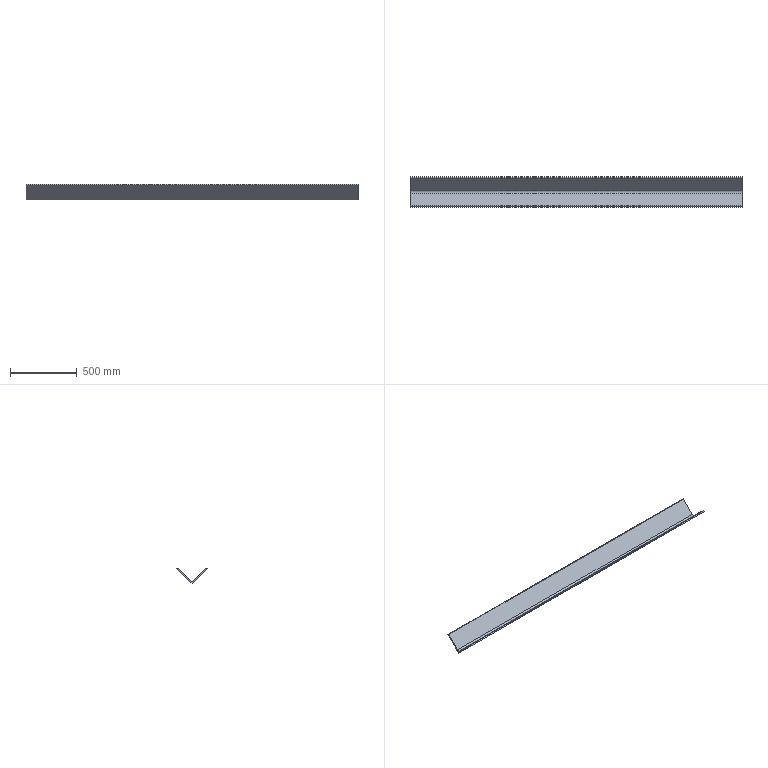Part | STEP file | Angle steel L160X60X10-2484_Default<As machined> | 1 solid | 13 faces | box 2484 x 226.274 x 118.827 mm | volume 7825020 mm3 | plane 8 | cylinder 5 | commonest cylinder face diameters 6.667 x4 32 x1
STEP:
#1=CARTESIAN_POINT('',(0.,0.,0.));
#2=DIRECTION('',(0.,0.,1.));
#3=DIRECTION('',(1.,0.,0.));
#4=AXIS2_PLACEMENT_3D('',#1,#2,#3);
#5=CARTESIAN_POINT('',(1242.,-106.066,118.827));
#6=VERTEX_POINT('',#5);
#7=CARTESIAN_POINT('',(1242.,-108.423,117.851));
#8=VERTEX_POINT('',#7);
#9=CARTESIAN_POINT('',(1242.,-106.066,115.494));
#10=DIRECTION('',(1.,0.,0.));
#11=DIRECTION('',(0.,0.,1.));
#12=AXIS2_PLACEMENT_3D('',#9,#10,#11);
#13=CIRCLE('',#12,3.333);
#14=CARTESIAN_POINT('',(1242.,-106.066,115.494));
#15=DIRECTION('',(-1.,0.,0.));
#16=DIRECTION('',(0.,0.,1.));
#17=AXIS2_PLACEMENT_3D('',#14,#15,#16);
#18=CYLINDRICAL_SURFACE('',#17,3.333);
#19=CARTESIAN_POINT('',(6.283,0.));
#20=DIRECTION('',(-1.,0.));
#21=VECTOR('',#20,1.);
#22=LINE('',#19,#21);
#23=(GEOMETRIC_REPRESENTATION_CONTEXT(2)PARAMETRIC_REPRESENTATION_CONTEXT()REPRESENTATION_CONTEXT('',''));
#24=DEFINITIONAL_REPRESENTATION('',(#22),#23);
#25=PCURVE('',#18,#24);
#26=CARTESIAN_POINT('',(1242.,-106.066,115.494));
#27=DIRECTION('',(-1.,0.,0.));
#28=DIRECTION('',(0.,0.,1.));
#29=AXIS2_PLACEMENT_3D('',#26,#27,#28);
#30=PLANE('',#29);
#31=CARTESIAN_POINT('',(3.333,0.));
#32=CARTESIAN_POINT('',(3.333,-5.774));
#33=CARTESIAN_POINT('',(-1.667,-2.887));
#34=CARTESIAN_POINT('',(-6.667,0.));
#35=CARTESIAN_POINT('',(-1.667,2.887));
#36=CARTESIAN_POINT('',(3.333,5.774));
#37=CARTESIAN_POINT('',(3.333,0.));
#38=(BOUNDED_CURVE()B_SPLINE_CURVE(2,(#31,#32,#33,#34,#35,#36,#37),.UNSPECIFIED.,.T.,.F.)B_SPLINE_CURVE_WITH_KNOTS((1,2,2,2,2,1),(-2.094,0.,2.094,4.189,6.283,8.378),.UNSPECIFIED.)CURVE()GEOMETRIC_REPRESENTATION_ITEM()RATIONAL_B_SPLINE_CURVE((1.,0.5,1.,0.5,1.,0.5,1.))REPRESENTATION_ITEM(''));
#39=(GEOMETRIC_REPRESENTATION_CONTEXT(2)PARAMETRIC_REPRESENTATION_CONTEXT()REPRESENTATION_CONTEXT('',''));
#40=DEFINITIONAL_REPRESENTATION('',(#38),#39);
#41=PCURVE('',#30,#40);
#42=SURFACE_CURVE('',#13,(#25,#41),.PCURVE_S1.);
#43=EDGE_CURVE('',#6,#8,#42,.T.);
#44=ORIENTED_EDGE('',*,*,#43,.F.);
#45=CARTESIAN_POINT('',(-1242.,-106.066,118.827));
#46=VERTEX_POINT('',#45);
#47=CARTESIAN_POINT('',(1242.,-106.066,118.827));
#48=DIRECTION('',(-1.,0.,0.));
#49=VECTOR('',#48,1.);
#50=LINE('',#47,#49);
#51=CARTESIAN_POINT('',(6.283,0.));
#52=DIRECTION('',(0.,1.));
#53=VECTOR('',#52,1.);
#54=LINE('',#51,#53);
#55=(GEOMETRIC_REPRESENTATION_CONTEXT(2)PARAMETRIC_REPRESENTATION_CONTEXT()REPRESENTATION_CONTEXT('',''));
#56=DEFINITIONAL_REPRESENTATION('',(#54),#55);
#57=PCURVE('',#18,#56);
#58=CARTESIAN_POINT('',(1242.,-106.066,115.494));
#59=DIRECTION('',(-1.,0.,0.));
#60=DIRECTION('',(0.,0.,1.));
#61=AXIS2_PLACEMENT_3D('',#58,#59,#60);
#62=CYLINDRICAL_SURFACE('',#61,3.333);
#63=CARTESIAN_POINT('',(0.,0.));
#64=DIRECTION('',(0.,1.));
#65=VECTOR('',#64,1.);
#66=LINE('',#63,#65);
#67=(GEOMETRIC_REPRESENTATION_CONTEXT(2)PARAMETRIC_REPRESENTATION_CONTEXT()REPRESENTATION_CONTEXT('',''));
#68=DEFINITIONAL_REPRESENTATION('',(#66),#67);
#69=PCURVE('',#62,#68);
#70=SURFACE_CURVE('',#50,(#57,#69),.PCURVE_S1.);
#71=EDGE_CURVE('',#6,#46,#70,.T.);
#72=ORIENTED_EDGE('',*,*,#71,.T.);
#73=CARTESIAN_POINT('',(-1242.,-108.423,117.851));
#74=VERTEX_POINT('',#73);
#75=CARTESIAN_POINT('',(-1242.,-106.066,115.494));
#76=DIRECTION('',(1.,0.,0.));
#77=DIRECTION('',(0.,0.,1.));
#78=AXIS2_PLACEMENT_3D('',#75,#76,#77);
#79=CIRCLE('',#78,3.333);
#80=CARTESIAN_POINT('',(6.283,2484.));
#81=DIRECTION('',(-1.,0.));
#82=VECTOR('',#81,1.);
#83=LINE('',#80,#82);
#84=(GEOMETRIC_REPRESENTATION_CONTEXT(2)PARAMETRIC_REPRESENTATION_CONTEXT()REPRESENTATION_CONTEXT('',''));
#85=DEFINITIONAL_REPRESENTATION('',(#83),#84);
#86=PCURVE('',#18,#85);
#87=CARTESIAN_POINT('',(-1242.,-106.066,115.494));
#88=DIRECTION('',(-1.,0.,0.));
#89=DIRECTION('',(0.,0.,1.));
#90=AXIS2_PLACEMENT_3D('',#87,#88,#89);
#91=PLANE('',#90);
#92=CARTESIAN_POINT('',(3.333,0.));
#93=CARTESIAN_POINT('',(3.333,-5.774));
#94=CARTESIAN_POINT('',(-1.667,-2.887));
#95=CARTESIAN_POINT('',(-6.667,0.));
#96=CARTESIAN_POINT('',(-1.667,2.887));
#97=CARTESIAN_POINT('',(3.333,5.774));
#98=CARTESIAN_POINT('',(3.333,0.));
#99=(BOUNDED_CURVE()B_SPLINE_CURVE(2,(#92,#93,#94,#95,#96,#97,#98),.UNSPECIFIED.,.T.,.F.)B_SPLINE_CURVE_WITH_KNOTS((1,2,2,2,2,1),(-2.094,0.,2.094,4.189,6.283,8.378),.UNSPECIFIED.)CURVE()GEOMETRIC_REPRESENTATION_ITEM()RATIONAL_B_SPLINE_CURVE((1.,0.5,1.,0.5,1.,0.5,1.))REPRESENTATION_ITEM(''));
#100=(GEOMETRIC_REPRESENTATION_CONTEXT(2)PARAMETRIC_REPRESENTATION_CONTEXT()REPRESENTATION_CONTEXT('',''));
#101=DEFINITIONAL_REPRESENTATION('',(#99),#100);
#102=PCURVE('',#91,#101);
#103=SURFACE_CURVE('',#79,(#86,#102),.PCURVE_S1.);
#104=EDGE_CURVE('',#46,#74,#103,.T.);
#105=ORIENTED_EDGE('',*,*,#104,.T.);
#106=CARTESIAN_POINT('',(1242.,-108.423,117.851));
#107=DIRECTION('',(-1.,0.,0.));
#108=VECTOR('',#107,1.);
#109=LINE('',#106,#108);
#110=CARTESIAN_POINT('',(5.498,0.));
#111=DIRECTION('',(0.,1.));
#112=VECTOR('',#111,1.);
#113=LINE('',#110,#112);
#114=(GEOMETRIC_REPRESENTATION_CONTEXT(2)PARAMETRIC_REPRESENTATION_CONTEXT()REPRESENTATION_CONTEXT('',''));
#115=DEFINITIONAL_REPRESENTATION('',(#113),#114);
#116=PCURVE('',#18,#115);
#117=CARTESIAN_POINT('',(1242.,-113.137,113.137));
#118=DIRECTION('',(0.,0.7071,-0.7071));
#119=DIRECTION('',(0.,0.7071,0.7071));
#120=AXIS2_PLACEMENT_3D('',#117,#118,#119);
#121=PLANE('',#120);
#122=CARTESIAN_POINT('',(6.667,0.));
#123=DIRECTION('',(0.,-1.));
#124=VECTOR('',#123,1.);
#125=LINE('',#122,#124);
#126=(GEOMETRIC_REPRESENTATION_CONTEXT(2)PARAMETRIC_REPRESENTATION_CONTEXT()REPRESENTATION_CONTEXT('',''));
#127=DEFINITIONAL_REPRESENTATION('',(#125),#126);
#128=PCURVE('',#121,#127);
#129=SURFACE_CURVE('',#109,(#116,#128),.PCURVE_S1.);
#130=EDGE_CURVE('',#8,#74,#129,.T.);
#131=ORIENTED_EDGE('',*,*,#130,.F.);
#132=EDGE_LOOP('',(#44,#72,#105,#131));
#133=FACE_BOUND('',#132,.T.);
#134=ADVANCED_FACE('',(#133),#18,.T.);
#135=CARTESIAN_POINT('',(1242.,106.066,118.827));
#136=VERTEX_POINT('',#135);
#137=CARTESIAN_POINT('',(1242.,103.709,117.851));
#138=VERTEX_POINT('',#137);
#139=CARTESIAN_POINT('',(1242.,106.066,115.494));
#140=DIRECTION('',(1.,0.,0.));
#141=DIRECTION('',(0.,0.,-1.));
#142=AXIS2_PLACEMENT_3D('',#139,#140,#141);
#143=CIRCLE('',#142,3.333);
#144=CARTESIAN_POINT('',(1242.,106.066,115.494));
#145=DIRECTION('',(-1.,0.,0.));
#146=DIRECTION('',(0.,0.,1.));
#147=AXIS2_PLACEMENT_3D('',#144,#145,#146);
#148=CYLINDRICAL_SURFACE('',#147,3.333);
#149=CARTESIAN_POINT('',(9.425,0.));
#150=DIRECTION('',(-1.,0.));
#151=VECTOR('',#150,1.);
#152=LINE('',#149,#151);
#153=(GEOMETRIC_REPRESENTATION_CONTEXT(2)PARAMETRIC_REPRESENTATION_CONTEXT()REPRESENTATION_CONTEXT('',''));
#154=DEFINITIONAL_REPRESENTATION('',(#152),#153);
#155=PCURVE('',#148,#154);
#156=CARTESIAN_POINT('',(-3.333,212.132));
#157=CARTESIAN_POINT('',(-3.333,217.906));
#158=CARTESIAN_POINT('',(1.667,215.019));
#159=CARTESIAN_POINT('',(6.667,212.132));
#160=CARTESIAN_POINT('',(1.667,209.245));
#161=CARTESIAN_POINT('',(-3.333,206.359));
#162=CARTESIAN_POINT('',(-3.333,212.132));
#163=(BOUNDED_CURVE()B_SPLINE_CURVE(2,(#156,#157,#158,#159,#160,#161,#162),.UNSPECIFIED.,.T.,.F.)B_SPLINE_CURVE_WITH_KNOTS((1,2,2,2,2,1),(-2.094,0.,2.094,4.189,6.283,8.378),.UNSPECIFIED.)CURVE()GEOMETRIC_REPRESENTATION_ITEM()RATIONAL_B_SPLINE_CURVE((1.,0.5,1.,0.5,1.,0.5,1.))REPRESENTATION_ITEM(''));
#164=(GEOMETRIC_REPRESENTATION_CONTEXT(2)PARAMETRIC_REPRESENTATION_CONTEXT()REPRESENTATION_CONTEXT('',''));
#165=DEFINITIONAL_REPRESENTATION('',(#163),#164);
#166=PCURVE('',#30,#165);
#167=SURFACE_CURVE('',#143,(#155,#166),.PCURVE_S1.);
#168=EDGE_CURVE('',#136,#138,#167,.T.);
#169=ORIENTED_EDGE('',*,*,#168,.F.);
#170=CARTESIAN_POINT('',(-1242.,106.066,118.827));
#171=VERTEX_POINT('',#170);
#172=CARTESIAN_POINT('',(1242.,106.066,118.827));
#173=DIRECTION('',(-1.,0.,0.));
#174=VECTOR('',#173,1.);
#175=LINE('',#172,#174);
#176=CARTESIAN_POINT('',(6.283,0.));
#177=DIRECTION('',(0.,1.));
#178=VECTOR('',#177,1.);
#179=LINE('',#176,#178);
#180=(GEOMETRIC_REPRESENTATION_CONTEXT(2)PARAMETRIC_REPRESENTATION_CONTEXT()REPRESENTATION_CONTEXT('',''));
#181=DEFINITIONAL_REPRESENTATION('',(#179),#180);
#182=PCURVE('',#148,#181);
#183=CARTESIAN_POINT('',(1242.,106.066,115.494));
#184=DIRECTION('',(-1.,0.,0.));
#185=DIRECTION('',(0.,0.,1.));
#186=AXIS2_PLACEMENT_3D('',#183,#184,#185);
#187=CYLINDRICAL_SURFACE('',#186,3.333);
#188=CARTESIAN_POINT('',(0.,0.));
#189=DIRECTION('',(0.,1.));
#190=VECTOR('',#189,1.);
#191=LINE('',#188,#190);
#192=(GEOMETRIC_REPRESENTATION_CONTEXT(2)PARAMETRIC_REPRESENTATION_CONTEXT()REPRESENTATION_CONTEXT('',''));
#193=DEFINITIONAL_REPRESENTATION('',(#191),#192);
#194=PCURVE('',#187,#193);
#195=SURFACE_CURVE('',#175,(#182,#194),.PCURVE_S1.);
#196=EDGE_CURVE('',#136,#171,#195,.T.);
#197=ORIENTED_EDGE('',*,*,#196,.T.);
#198=CARTESIAN_POINT('',(-1242.,103.709,117.851));
#199=VERTEX_POINT('',#198);
#200=CARTESIAN_POINT('',(-1242.,106.066,115.494));
#201=DIRECTION('',(1.,0.,0.));
#202=DIRECTION('',(0.,0.,-1.));
#203=AXIS2_PLACEMENT_3D('',#200,#201,#202);
#204=CIRCLE('',#203,3.333);
#205=CARTESIAN_POINT('',(9.425,2484.));
#206=DIRECTION('',(-1.,0.));
#207=VECTOR('',#206,1.);
#208=LINE('',#205,#207);
#209=(GEOMETRIC_REPRESENTATION_CONTEXT(2)PARAMETRIC_REPRESENTATION_CONTEXT()REPRESENTATION_CONTEXT('',''));
#210=DEFINITIONAL_REPRESENTATION('',(#208),#209);
#211=PCURVE('',#148,#210);
#212=CARTESIAN_POINT('',(-3.333,212.132));
#213=CARTESIAN_POINT('',(-3.333,217.906));
#214=CARTESIAN_POINT('',(1.667,215.019));
#215=CARTESIAN_POINT('',(6.667,212.132));
#216=CARTESIAN_POINT('',(1.667,209.245));
#217=CARTESIAN_POINT('',(-3.333,206.359));
#218=CARTESIAN_POINT('',(-3.333,212.132));
#219=(BOUNDED_CURVE()B_SPLINE_CURVE(2,(#212,#213,#214,#215,#216,#217,#218),.UNSPECIFIED.,.T.,.F.)B_SPLINE_CURVE_WITH_KNOTS((1,2,2,2,2,1),(-2.094,0.,2.094,4.189,6.283,8.378),.UNSPECIFIED.)CURVE()GEOMETRIC_REPRESENTATION_ITEM()RATIONAL_B_SPLINE_CURVE((1.,0.5,1.,0.5,1.,0.5,1.))REPRESENTATION_ITEM(''));
#220=(GEOMETRIC_REPRESENTATION_CONTEXT(2)PARAMETRIC_REPRESENTATION_CONTEXT()REPRESENTATION_CONTEXT('',''));
#221=DEFINITIONAL_REPRESENTATION('',(#219),#220);
#222=PCURVE('',#91,#221);
#223=SURFACE_CURVE('',#204,(#211,#222),.PCURVE_S1.);
#224=EDGE_CURVE('',#171,#199,#223,.T.);
#225=ORIENTED_EDGE('',*,*,#224,.T.);
#226=CARTESIAN_POINT('',(1242.,103.709,117.851));
#227=DIRECTION('',(-1.,0.,0.));
#228=VECTOR('',#227,1.);
#229=LINE('',#226,#228);
#230=CARTESIAN_POINT('',(5.498,0.));
#231=DIRECTION('',(0.,1.));
#232=VECTOR('',#231,1.);
#233=LINE('',#230,#232);
#234=(GEOMETRIC_REPRESENTATION_CONTEXT(2)PARAMETRIC_REPRESENTATION_CONTEXT()REPRESENTATION_CONTEXT('',''));
#235=DEFINITIONAL_REPRESENTATION('',(#233),#234);
#236=PCURVE('',#148,#235);
#237=CARTESIAN_POINT('',(1242.,11.314,25.456));
#238=DIRECTION('',(0.,0.7071,-0.7071));
#239=DIRECTION('',(0.,0.7071,0.7071));
#240=AXIS2_PLACEMENT_3D('',#237,#238,#239);
#241=PLANE('',#240);
#242=CARTESIAN_POINT('',(130.667,0.));
#243=DIRECTION('',(0.,-1.));
#244=VECTOR('',#243,1.);
#245=LINE('',#242,#244);
#246=(GEOMETRIC_REPRESENTATION_CONTEXT(2)PARAMETRIC_REPRESENTATION_CONTEXT()REPRESENTATION_CONTEXT('',''));
#247=DEFINITIONAL_REPRESENTATION('',(#245),#246);
#248=PCURVE('',#241,#247);
#249=SURFACE_CURVE('',#229,(#236,#248),.PCURVE_S1.);
#250=EDGE_CURVE('',#138,#199,#249,.T.);
#251=ORIENTED_EDGE('',*,*,#250,.F.);
#252=EDGE_LOOP('',(#169,#197,#225,#251));
#253=FACE_BOUND('',#252,.T.);
#254=ADVANCED_FACE('',(#253),#148,.T.);
#255=CARTESIAN_POINT('',(-1242.,0.,0.));
#256=VERTEX_POINT('',#255);
#257=CARTESIAN_POINT('',(-1242.,113.137,113.137));
#258=VERTEX_POINT('',#257);
#259=CARTESIAN_POINT('',(-1242.,113.137,113.137));
#260=DIRECTION('',(0.,0.7071,0.7071));
#261=VECTOR('',#260,1.);
#262=LINE('',#259,#261);
#263=CARTESIAN_POINT('',(1242.,113.137,113.137));
#264=DIRECTION('',(0.,-0.7071,0.7071));
#265=DIRECTION('',(0.,-0.7071,-0.7071));
#266=AXIS2_PLACEMENT_3D('',#263,#264,#265);
#267=PLANE('',#266);
#268=CARTESIAN_POINT('',(0.,-2484.));
#269=DIRECTION('',(-1.,0.));
#270=VECTOR('',#269,1.);
#271=LINE('',#268,#270);
#272=(GEOMETRIC_REPRESENTATION_CONTEXT(2)PARAMETRIC_REPRESENTATION_CONTEXT()REPRESENTATION_CONTEXT('',''));
#273=DEFINITIONAL_REPRESENTATION('',(#271),#272);
#274=PCURVE('',#267,#273);
#275=CARTESIAN_POINT('',(-2.357,219.203));
#276=DIRECTION('',(0.7071,0.7071));
#277=VECTOR('',#276,1.);
#278=LINE('',#275,#277);
#279=(GEOMETRIC_REPRESENTATION_CONTEXT(2)PARAMETRIC_REPRESENTATION_CONTEXT()REPRESENTATION_CONTEXT('',''));
#280=DEFINITIONAL_REPRESENTATION('',(#278),#279);
#281=PCURVE('',#91,#280);
#282=SURFACE_CURVE('',#262,(#274,#281),.PCURVE_S1.);
#283=EDGE_CURVE('',#256,#258,#282,.T.);
#284=ORIENTED_EDGE('',*,*,#283,.T.);
#285=CARTESIAN_POINT('',(1242.,113.137,113.137));
#286=VERTEX_POINT('',#285);
#287=CARTESIAN_POINT('',(1242.,113.137,113.137));
#288=DIRECTION('',(-1.,0.,0.));
#289=VECTOR('',#288,1.);
#290=LINE('',#287,#289);
#291=CARTESIAN_POINT('',(0.,0.));
#292=DIRECTION('',(0.,-1.));
#293=VECTOR('',#292,1.);
#294=LINE('',#291,#293);
#295=(GEOMETRIC_REPRESENTATION_CONTEXT(2)PARAMETRIC_REPRESENTATION_CONTEXT()REPRESENTATION_CONTEXT('',''));
#296=DEFINITIONAL_REPRESENTATION('',(#294),#295);
#297=PCURVE('',#267,#296);
#298=CARTESIAN_POINT('',(1242.,113.137,113.137));
#299=DIRECTION('',(0.,-0.7071,-0.7071));
#300=DIRECTION('',(0.,0.7071,-0.7071));
#301=AXIS2_PLACEMENT_3D('',#298,#299,#300);
#302=PLANE('',#301);
#303=CARTESIAN_POINT('',(0.,0.));
#304=DIRECTION('',(0.,-1.));
#305=VECTOR('',#304,1.);
#306=LINE('',#303,#305);
#307=(GEOMETRIC_REPRESENTATION_CONTEXT(2)PARAMETRIC_REPRESENTATION_CONTEXT()REPRESENTATION_CONTEXT('',''));
#308=DEFINITIONAL_REPRESENTATION('',(#306),#307);
#309=PCURVE('',#302,#308);
#310=SURFACE_CURVE('',#290,(#297,#309),.PCURVE_S1.);
#311=EDGE_CURVE('',#286,#258,#310,.T.);
#312=ORIENTED_EDGE('',*,*,#311,.F.);
#313=CARTESIAN_POINT('',(1242.,0.,0.));
#314=VERTEX_POINT('',#313);
#315=CARTESIAN_POINT('',(1242.,113.137,113.137));
#316=DIRECTION('',(0.,0.7071,0.7071));
#317=VECTOR('',#316,1.);
#318=LINE('',#315,#317);
#319=CARTESIAN_POINT('',(0.,0.));
#320=DIRECTION('',(-1.,0.));
#321=VECTOR('',#320,1.);
#322=LINE('',#319,#321);
#323=(GEOMETRIC_REPRESENTATION_CONTEXT(2)PARAMETRIC_REPRESENTATION_CONTEXT()REPRESENTATION_CONTEXT('',''));
#324=DEFINITIONAL_REPRESENTATION('',(#322),#323);
#325=PCURVE('',#267,#324);
#326=CARTESIAN_POINT('',(-2.357,219.203));
#327=DIRECTION('',(0.7071,0.7071));
#328=VECTOR('',#327,1.);
#329=LINE('',#326,#328);
#330=(GEOMETRIC_REPRESENTATION_CONTEXT(2)PARAMETRIC_REPRESENTATION_CONTEXT()REPRESENTATION_CONTEXT('',''));
#331=DEFINITIONAL_REPRESENTATION('',(#329),#330);
#332=PCURVE('',#30,#331);
#333=SURFACE_CURVE('',#318,(#325,#332),.PCURVE_S1.);
#334=EDGE_CURVE('',#314,#286,#333,.T.);
#335=ORIENTED_EDGE('',*,*,#334,.F.);
#336=CARTESIAN_POINT('',(1242.,0.,0.));
#337=DIRECTION('',(-1.,0.,0.));
#338=VECTOR('',#337,1.);
#339=LINE('',#336,#338);
#340=CARTESIAN_POINT('',(160.,0.));
#341=DIRECTION('',(0.,-1.));
#342=VECTOR('',#341,1.);
#343=LINE('',#340,#342);
#344=(GEOMETRIC_REPRESENTATION_CONTEXT(2)PARAMETRIC_REPRESENTATION_CONTEXT()REPRESENTATION_CONTEXT('',''));
#345=DEFINITIONAL_REPRESENTATION('',(#343),#344);
#346=PCURVE('',#267,#345);
#347=CARTESIAN_POINT('',(1242.,0.,0.));
#348=DIRECTION('',(0.,0.7071,0.7071));
#349=DIRECTION('',(0.,-0.7071,0.7071));
#350=AXIS2_PLACEMENT_3D('',#347,#348,#349);
#351=PLANE('',#350);
#352=CARTESIAN_POINT('',(0.,0.));
#353=DIRECTION('',(0.,-1.));
#354=VECTOR('',#353,1.);
#355=LINE('',#352,#354);
#356=(GEOMETRIC_REPRESENTATION_CONTEXT(2)PARAMETRIC_REPRESENTATION_CONTEXT()REPRESENTATION_CONTEXT('',''));
#357=DEFINITIONAL_REPRESENTATION('',(#355),#356);
#358=PCURVE('',#351,#357);
#359=SURFACE_CURVE('',#339,(#346,#358),.PCURVE_S1.);
#360=EDGE_CURVE('',#314,#256,#359,.T.);
#361=ORIENTED_EDGE('',*,*,#360,.T.);
#362=EDGE_LOOP('',(#284,#312,#335,#361));
#363=FACE_BOUND('',#362,.T.);
#364=ADVANCED_FACE('',(#363),#267,.F.);
#365=CARTESIAN_POINT('',(-1242.,108.423,117.851));
#366=VERTEX_POINT('',#365);
#367=CARTESIAN_POINT('',(-1242.,113.137,113.137));
#368=DIRECTION('',(0.,-0.7071,0.7071));
#369=VECTOR('',#368,1.);
#370=LINE('',#367,#369);
#371=CARTESIAN_POINT('',(0.,-2484.));
#372=DIRECTION('',(-1.,0.));
#373=VECTOR('',#372,1.);
#374=LINE('',#371,#373);
#375=(GEOMETRIC_REPRESENTATION_CONTEXT(2)PARAMETRIC_REPRESENTATION_CONTEXT()REPRESENTATION_CONTEXT('',''));
#376=DEFINITIONAL_REPRESENTATION('',(#374),#375);
#377=PCURVE('',#302,#376);
#378=CARTESIAN_POINT('',(-2.357,219.203));
#379=DIRECTION('',(0.7071,-0.7071));
#380=VECTOR('',#379,1.);
#381=LINE('',#378,#380);
#382=(GEOMETRIC_REPRESENTATION_CONTEXT(2)PARAMETRIC_REPRESENTATION_CONTEXT()REPRESENTATION_CONTEXT('',''));
#383=DEFINITIONAL_REPRESENTATION('',(#381),#382);
#384=PCURVE('',#91,#383);
#385=SURFACE_CURVE('',#370,(#377,#384),.PCURVE_S1.);
#386=EDGE_CURVE('',#258,#366,#385,.T.);
#387=ORIENTED_EDGE('',*,*,#386,.T.);
#388=CARTESIAN_POINT('',(1242.,108.423,117.851));
#389=VERTEX_POINT('',#388);
#390=CARTESIAN_POINT('',(1242.,108.423,117.851));
#391=DIRECTION('',(-1.,0.,0.));
#392=VECTOR('',#391,1.);
#393=LINE('',#390,#392);
#394=CARTESIAN_POINT('',(-6.667,0.));
#395=DIRECTION('',(0.,-1.));
#396=VECTOR('',#395,1.);
#397=LINE('',#394,#396);
#398=(GEOMETRIC_REPRESENTATION_CONTEXT(2)PARAMETRIC_REPRESENTATION_CONTEXT()REPRESENTATION_CONTEXT('',''));
#399=DEFINITIONAL_REPRESENTATION('',(#397),#398);
#400=PCURVE('',#302,#399);
#401=CARTESIAN_POINT('',(0.7854,0.));
#402=DIRECTION('',(0.,1.));
#403=VECTOR('',#402,1.);
#404=LINE('',#401,#403);
#405=(GEOMETRIC_REPRESENTATION_CONTEXT(2)PARAMETRIC_REPRESENTATION_CONTEXT()REPRESENTATION_CONTEXT('',''));
#406=DEFINITIONAL_REPRESENTATION('',(#404),#405);
#407=PCURVE('',#187,#406);
#408=SURFACE_CURVE('',#393,(#400,#407),.PCURVE_S1.);
#409=EDGE_CURVE('',#389,#366,#408,.T.);
#410=ORIENTED_EDGE('',*,*,#409,.F.);
#411=CARTESIAN_POINT('',(1242.,113.137,113.137));
#412=DIRECTION('',(0.,-0.7071,0.7071));
#413=VECTOR('',#412,1.);
#414=LINE('',#411,#413);
#415=CARTESIAN_POINT('',(0.,0.));
#416=DIRECTION('',(-1.,0.));
#417=VECTOR('',#416,1.);
#418=LINE('',#415,#417);
#419=(GEOMETRIC_REPRESENTATION_CONTEXT(2)PARAMETRIC_REPRESENTATION_CONTEXT()REPRESENTATION_CONTEXT('',''));
#420=DEFINITIONAL_REPRESENTATION('',(#418),#419);
#421=PCURVE('',#302,#420);
#422=CARTESIAN_POINT('',(-2.357,219.203));
#423=DIRECTION('',(0.7071,-0.7071));
#424=VECTOR('',#423,1.);
#425=LINE('',#422,#424);
#426=(GEOMETRIC_REPRESENTATION_CONTEXT(2)PARAMETRIC_REPRESENTATION_CONTEXT()REPRESENTATION_CONTEXT('',''));
#427=DEFINITIONAL_REPRESENTATION('',(#425),#426);
#428=PCURVE('',#30,#427);
#429=SURFACE_CURVE('',#414,(#421,#428),.PCURVE_S1.);
#430=EDGE_CURVE('',#286,#389,#429,.T.);
#431=ORIENTED_EDGE('',*,*,#430,.F.);
#432=ORIENTED_EDGE('',*,*,#311,.T.);
#433=EDGE_LOOP('',(#387,#410,#431,#432));
#434=FACE_BOUND('',#433,.T.);
#435=ADVANCED_FACE('',(#434),#302,.F.);
#436=ORIENTED_EDGE('',*,*,#196,.F.);
#437=CARTESIAN_POINT('',(1242.,106.066,115.494));
#438=DIRECTION('',(1.,0.,0.));
#439=DIRECTION('',(0.,0.,-1.));
#440=AXIS2_PLACEMENT_3D('',#437,#438,#439);
#441=CIRCLE('',#440,3.333);
#442=CARTESIAN_POINT('',(3.142,0.));
#443=DIRECTION('',(-1.,0.));
#444=VECTOR('',#443,1.);
#445=LINE('',#442,#444);
#446=(GEOMETRIC_REPRESENTATION_CONTEXT(2)PARAMETRIC_REPRESENTATION_CONTEXT()REPRESENTATION_CONTEXT('',''));
#447=DEFINITIONAL_REPRESENTATION('',(#445),#446);
#448=PCURVE('',#187,#447);
#449=CARTESIAN_POINT('',(-3.333,212.132));
#450=CARTESIAN_POINT('',(-3.333,217.906));
#451=CARTESIAN_POINT('',(1.667,215.019));
#452=CARTESIAN_POINT('',(6.667,212.132));
#453=CARTESIAN_POINT('',(1.667,209.245));
#454=CARTESIAN_POINT('',(-3.333,206.359));
#455=CARTESIAN_POINT('',(-3.333,212.132));
#456=(BOUNDED_CURVE()B_SPLINE_CURVE(2,(#449,#450,#451,#452,#453,#454,#455),.UNSPECIFIED.,.T.,.F.)B_SPLINE_CURVE_WITH_KNOTS((1,2,2,2,2,1),(-2.094,0.,2.094,4.189,6.283,8.378),.UNSPECIFIED.)CURVE()GEOMETRIC_REPRESENTATION_ITEM()RATIONAL_B_SPLINE_CURVE((1.,0.5,1.,0.5,1.,0.5,1.))REPRESENTATION_ITEM(''));
#457=(GEOMETRIC_REPRESENTATION_CONTEXT(2)PARAMETRIC_REPRESENTATION_CONTEXT()REPRESENTATION_CONTEXT('',''));
#458=DEFINITIONAL_REPRESENTATION('',(#456),#457);
#459=PCURVE('',#30,#458);
#460=SURFACE_CURVE('',#441,(#448,#459),.PCURVE_S1.);
#461=EDGE_CURVE('',#389,#136,#460,.T.);
#462=ORIENTED_EDGE('',*,*,#461,.F.);
#463=ORIENTED_EDGE('',*,*,#409,.T.);
#464=CARTESIAN_POINT('',(-1242.,106.066,115.494));
#465=DIRECTION('',(1.,0.,0.));
#466=DIRECTION('',(0.,0.,-1.));
#467=AXIS2_PLACEMENT_3D('',#464,#465,#466);
#468=CIRCLE('',#467,3.333);
#469=CARTESIAN_POINT('',(3.142,2484.));
#470=DIRECTION('',(-1.,0.));
#471=VECTOR('',#470,1.);
#472=LINE('',#469,#471);
#473=(GEOMETRIC_REPRESENTATION_CONTEXT(2)PARAMETRIC_REPRESENTATION_CONTEXT()REPRESENTATION_CONTEXT('',''));
#474=DEFINITIONAL_REPRESENTATION('',(#472),#473);
#475=PCURVE('',#187,#474);
#476=CARTESIAN_POINT('',(-3.333,212.132));
#477=CARTESIAN_POINT('',(-3.333,217.906));
#478=CARTESIAN_POINT('',(1.667,215.019));
#479=CARTESIAN_POINT('',(6.667,212.132));
#480=CARTESIAN_POINT('',(1.667,209.245));
#481=CARTESIAN_POINT('',(-3.333,206.359));
#482=CARTESIAN_POINT('',(-3.333,212.132));
#483=(BOUNDED_CURVE()B_SPLINE_CURVE(2,(#476,#477,#478,#479,#480,#481,#482),.UNSPECIFIED.,.T.,.F.)B_SPLINE_CURVE_WITH_KNOTS((1,2,2,2,2,1),(-2.094,0.,2.094,4.189,6.283,8.378),.UNSPECIFIED.)CURVE()GEOMETRIC_REPRESENTATION_ITEM()RATIONAL_B_SPLINE_CURVE((1.,0.5,1.,0.5,1.,0.5,1.))REPRESENTATION_ITEM(''));
#484=(GEOMETRIC_REPRESENTATION_CONTEXT(2)PARAMETRIC_REPRESENTATION_CONTEXT()REPRESENTATION_CONTEXT('',''));
#485=DEFINITIONAL_REPRESENTATION('',(#483),#484);
#486=PCURVE('',#91,#485);
#487=SURFACE_CURVE('',#468,(#475,#486),.PCURVE_S1.);
#488=EDGE_CURVE('',#366,#171,#487,.T.);
#489=ORIENTED_EDGE('',*,*,#488,.T.);
#490=EDGE_LOOP('',(#436,#462,#463,#489));
#491=FACE_BOUND('',#490,.T.);
#492=ADVANCED_FACE('',(#491),#187,.T.);
#493=CARTESIAN_POINT('',(-1242.,11.314,25.456));
#494=VERTEX_POINT('',#493);
#495=CARTESIAN_POINT('',(-1242.,11.314,25.456));
#496=DIRECTION('',(0.,-0.7071,-0.7071));
#497=VECTOR('',#496,1.);
#498=LINE('',#495,#497);
#499=CARTESIAN_POINT('',(0.,-2484.));
#500=DIRECTION('',(-1.,0.));
#501=VECTOR('',#500,1.);
#502=LINE('',#499,#501);
#503=(GEOMETRIC_REPRESENTATION_CONTEXT(2)PARAMETRIC_REPRESENTATION_CONTEXT()REPRESENTATION_CONTEXT('',''));
#504=DEFINITIONAL_REPRESENTATION('',(#502),#503);
#505=PCURVE('',#241,#504);
#506=CARTESIAN_POINT('',(-90.038,117.38));
#507=DIRECTION('',(-0.7071,-0.7071));
#508=VECTOR('',#507,1.);
#509=LINE('',#506,#508);
#510=(GEOMETRIC_REPRESENTATION_CONTEXT(2)PARAMETRIC_REPRESENTATION_CONTEXT()REPRESENTATION_CONTEXT('',''));
#511=DEFINITIONAL_REPRESENTATION('',(#509),#510);
#512=PCURVE('',#91,#511);
#513=SURFACE_CURVE('',#498,(#505,#512),.PCURVE_S1.);
#514=EDGE_CURVE('',#199,#494,#513,.T.);
#515=ORIENTED_EDGE('',*,*,#514,.T.);
#516=CARTESIAN_POINT('',(1242.,11.314,25.456));
#517=VERTEX_POINT('',#516);
#518=CARTESIAN_POINT('',(1242.,11.314,25.456));
#519=DIRECTION('',(-1.,0.,0.));
#520=VECTOR('',#519,1.);
#521=LINE('',#518,#520);
#522=CARTESIAN_POINT('',(0.,0.));
#523=DIRECTION('',(0.,-1.));
#524=VECTOR('',#523,1.);
#525=LINE('',#522,#524);
#526=(GEOMETRIC_REPRESENTATION_CONTEXT(2)PARAMETRIC_REPRESENTATION_CONTEXT()REPRESENTATION_CONTEXT('',''));
#527=DEFINITIONAL_REPRESENTATION('',(#525),#526);
#528=PCURVE('',#241,#527);
#529=CARTESIAN_POINT('',(1242.,0.,36.77));
#530=DIRECTION('',(-1.,0.,0.));
#531=DIRECTION('',(0.,0.,1.));
#532=AXIS2_PLACEMENT_3D('',#529,#530,#531);
#533=CYLINDRICAL_SURFACE('',#532,16.);
#534=CARTESIAN_POINT('',(2.356,0.));
#535=DIRECTION('',(0.,1.));
#536=VECTOR('',#535,1.);
#537=LINE('',#534,#536);
#538=(GEOMETRIC_REPRESENTATION_CONTEXT(2)PARAMETRIC_REPRESENTATION_CONTEXT()REPRESENTATION_CONTEXT('',''));
#539=DEFINITIONAL_REPRESENTATION('',(#537),#538);
#540=PCURVE('',#533,#539);
#541=SURFACE_CURVE('',#521,(#528,#540),.PCURVE_S1.);
#542=EDGE_CURVE('',#517,#494,#541,.T.);
#543=ORIENTED_EDGE('',*,*,#542,.F.);
#544=CARTESIAN_POINT('',(1242.,11.314,25.456));
#545=DIRECTION('',(0.,-0.7071,-0.7071));
#546=VECTOR('',#545,1.);
#547=LINE('',#544,#546);
#548=CARTESIAN_POINT('',(0.,0.));
#549=DIRECTION('',(-1.,0.));
#550=VECTOR('',#549,1.);
#551=LINE('',#548,#550);
#552=(GEOMETRIC_REPRESENTATION_CONTEXT(2)PARAMETRIC_REPRESENTATION_CONTEXT()REPRESENTATION_CONTEXT('',''));
#553=DEFINITIONAL_REPRESENTATION('',(#551),#552);
#554=PCURVE('',#241,#553);
#555=CARTESIAN_POINT('',(-90.038,117.38));
#556=DIRECTION('',(-0.7071,-0.7071));
#557=VECTOR('',#556,1.);
#558=LINE('',#555,#557);
#559=(GEOMETRIC_REPRESENTATION_CONTEXT(2)PARAMETRIC_REPRESENTATION_CONTEXT()REPRESENTATION_CONTEXT('',''));
#560=DEFINITIONAL_REPRESENTATION('',(#558),#559);
#561=PCURVE('',#30,#560);
#562=SURFACE_CURVE('',#547,(#554,#561),.PCURVE_S1.);
#563=EDGE_CURVE('',#138,#517,#562,.T.);
#564=ORIENTED_EDGE('',*,*,#563,.F.);
#565=ORIENTED_EDGE('',*,*,#250,.T.);
#566=EDGE_LOOP('',(#515,#543,#564,#565));
#567=FACE_BOUND('',#566,.T.);
#568=ADVANCED_FACE('',(#567),#241,.F.);
#569=ORIENTED_EDGE('',*,*,#542,.F.);
#570=CARTESIAN_POINT('',(1242.,-11.314,25.456));
#571=VERTEX_POINT('',#570);
#572=CARTESIAN_POINT('',(1242.,0.,36.77));
#573=DIRECTION('',(-1.,0.,0.));
#574=DIRECTION('',(0.,0.,1.));
#575=AXIS2_PLACEMENT_3D('',#572,#573,#574);
#576=CIRCLE('',#575,16.);
#577=CARTESIAN_POINT('',(0.,0.));
#578=DIRECTION('',(1.,0.));
#579=VECTOR('',#578,1.);
#580=LINE('',#577,#579);
#581=(GEOMETRIC_REPRESENTATION_CONTEXT(2)PARAMETRIC_REPRESENTATION_CONTEXT()REPRESENTATION_CONTEXT('',''));
#582=DEFINITIONAL_REPRESENTATION('',(#580),#581);
#583=PCURVE('',#533,#582);
#584=CARTESIAN_POINT('',(-78.725,106.066));
#585=DIRECTION('',(1.,0.));
#586=AXIS2_PLACEMENT_2D('',#584,#585);
#587=CIRCLE('',#586,16.);
#588=(GEOMETRIC_REPRESENTATION_CONTEXT(2)PARAMETRIC_REPRESENTATION_CONTEXT()REPRESENTATION_CONTEXT('',''));
#589=DEFINITIONAL_REPRESENTATION('',(#587),#588);
#590=PCURVE('',#30,#589);
#591=SURFACE_CURVE('',#576,(#583,#590),.PCURVE_S1.);
#592=EDGE_CURVE('',#517,#571,#591,.T.);
#593=ORIENTED_EDGE('',*,*,#592,.T.);
#594=CARTESIAN_POINT('',(-1242.,-11.314,25.456));
#595=VERTEX_POINT('',#594);
#596=CARTESIAN_POINT('',(1242.,-11.314,25.456));
#597=DIRECTION('',(-1.,0.,0.));
#598=VECTOR('',#597,1.);
#599=LINE('',#596,#598);
#600=CARTESIAN_POINT('',(3.927,0.));
#601=DIRECTION('',(0.,1.));
#602=VECTOR('',#601,1.);
#603=LINE('',#600,#602);
#604=(GEOMETRIC_REPRESENTATION_CONTEXT(2)PARAMETRIC_REPRESENTATION_CONTEXT()REPRESENTATION_CONTEXT('',''));
#605=DEFINITIONAL_REPRESENTATION('',(#603),#604);
#606=PCURVE('',#533,#605);
#607=CARTESIAN_POINT('',(1242.,-103.709,117.851));
#608=DIRECTION('',(0.,-0.7071,-0.7071));
#609=DIRECTION('',(0.,0.7071,-0.7071));
#610=AXIS2_PLACEMENT_3D('',#607,#608,#609);
#611=PLANE('',#610);
#612=CARTESIAN_POINT('',(130.667,0.));
#613=DIRECTION('',(0.,-1.));
#614=VECTOR('',#613,1.);
#615=LINE('',#612,#614);
#616=(GEOMETRIC_REPRESENTATION_CONTEXT(2)PARAMETRIC_REPRESENTATION_CONTEXT()REPRESENTATION_CONTEXT('',''));
#617=DEFINITIONAL_REPRESENTATION('',(#615),#616);
#618=PCURVE('',#611,#617);
#619=SURFACE_CURVE('',#599,(#606,#618),.PCURVE_S1.);
#620=EDGE_CURVE('',#571,#595,#619,.T.);
#621=ORIENTED_EDGE('',*,*,#620,.T.);
#622=CARTESIAN_POINT('',(-1242.,0.,36.77));
#623=DIRECTION('',(-1.,0.,0.));
#624=DIRECTION('',(0.,0.,1.));
#625=AXIS2_PLACEMENT_3D('',#622,#623,#624);
#626=CIRCLE('',#625,16.);
#627=CARTESIAN_POINT('',(0.,2484.));
#628=DIRECTION('',(1.,0.));
#629=VECTOR('',#628,1.);
#630=LINE('',#627,#629);
#631=(GEOMETRIC_REPRESENTATION_CONTEXT(2)PARAMETRIC_REPRESENTATION_CONTEXT()REPRESENTATION_CONTEXT('',''));
#632=DEFINITIONAL_REPRESENTATION('',(#630),#631);
#633=PCURVE('',#533,#632);
#634=CARTESIAN_POINT('',(-78.725,106.066));
#635=DIRECTION('',(1.,0.));
#636=AXIS2_PLACEMENT_2D('',#634,#635);
#637=CIRCLE('',#636,16.);
#638=(GEOMETRIC_REPRESENTATION_CONTEXT(2)PARAMETRIC_REPRESENTATION_CONTEXT()REPRESENTATION_CONTEXT('',''));
#639=DEFINITIONAL_REPRESENTATION('',(#637),#638);
#640=PCURVE('',#91,#639);
#641=SURFACE_CURVE('',#626,(#633,#640),.PCURVE_S1.);
#642=EDGE_CURVE('',#494,#595,#641,.T.);
#643=ORIENTED_EDGE('',*,*,#642,.F.);
#644=EDGE_LOOP('',(#569,#593,#621,#643));
#645=FACE_BOUND('',#644,.F.);
#646=ADVANCED_FACE('',(#645),#533,.F.);
#647=CARTESIAN_POINT('',(-1242.,-103.709,117.851));
#648=VERTEX_POINT('',#647);
#649=CARTESIAN_POINT('',(-1242.,-103.709,117.851));
#650=DIRECTION('',(0.,-0.7071,0.7071));
#651=VECTOR('',#650,1.);
#652=LINE('',#649,#651);
#653=CARTESIAN_POINT('',(0.,-2484.));
#654=DIRECTION('',(-1.,0.));
#655=VECTOR('',#654,1.);
#656=LINE('',#653,#655);
#657=(GEOMETRIC_REPRESENTATION_CONTEXT(2)PARAMETRIC_REPRESENTATION_CONTEXT()REPRESENTATION_CONTEXT('',''));
#658=DEFINITIONAL_REPRESENTATION('',(#656),#657);
#659=PCURVE('',#611,#658);
#660=CARTESIAN_POINT('',(2.357,2.357));
#661=DIRECTION('',(0.7071,-0.7071));
#662=VECTOR('',#661,1.);
#663=LINE('',#660,#662);
#664=(GEOMETRIC_REPRESENTATION_CONTEXT(2)PARAMETRIC_REPRESENTATION_CONTEXT()REPRESENTATION_CONTEXT('',''));
#665=DEFINITIONAL_REPRESENTATION('',(#663),#664);
#666=PCURVE('',#91,#665);
#667=SURFACE_CURVE('',#652,(#659,#666),.PCURVE_S1.);
#668=EDGE_CURVE('',#595,#648,#667,.T.);
#669=ORIENTED_EDGE('',*,*,#668,.T.);
#670=CARTESIAN_POINT('',(1242.,-103.709,117.851));
#671=VERTEX_POINT('',#670);
#672=CARTESIAN_POINT('',(1242.,-103.709,117.851));
#673=DIRECTION('',(-1.,0.,0.));
#674=VECTOR('',#673,1.);
#675=LINE('',#672,#674);
#676=CARTESIAN_POINT('',(0.,0.));
#677=DIRECTION('',(0.,-1.));
#678=VECTOR('',#677,1.);
#679=LINE('',#676,#678);
#680=(GEOMETRIC_REPRESENTATION_CONTEXT(2)PARAMETRIC_REPRESENTATION_CONTEXT()REPRESENTATION_CONTEXT('',''));
#681=DEFINITIONAL_REPRESENTATION('',(#679),#680);
#682=PCURVE('',#611,#681);
#683=CARTESIAN_POINT('',(0.7854,0.));
#684=DIRECTION('',(0.,1.));
#685=VECTOR('',#684,1.);
#686=LINE('',#683,#685);
#687=(GEOMETRIC_REPRESENTATION_CONTEXT(2)PARAMETRIC_REPRESENTATION_CONTEXT()REPRESENTATION_CONTEXT('',''));
#688=DEFINITIONAL_REPRESENTATION('',(#686),#687);
#689=PCURVE('',#62,#688);
#690=SURFACE_CURVE('',#675,(#682,#689),.PCURVE_S1.);
#691=EDGE_CURVE('',#671,#648,#690,.T.);
#692=ORIENTED_EDGE('',*,*,#691,.F.);
#693=CARTESIAN_POINT('',(1242.,-103.709,117.851));
#694=DIRECTION('',(0.,-0.7071,0.7071));
#695=VECTOR('',#694,1.);
#696=LINE('',#693,#695);
#697=CARTESIAN_POINT('',(0.,0.));
#698=DIRECTION('',(-1.,0.));
#699=VECTOR('',#698,1.);
#700=LINE('',#697,#699);
#701=(GEOMETRIC_REPRESENTATION_CONTEXT(2)PARAMETRIC_REPRESENTATION_CONTEXT()REPRESENTATION_CONTEXT('',''));
#702=DEFINITIONAL_REPRESENTATION('',(#700),#701);
#703=PCURVE('',#611,#702);
#704=CARTESIAN_POINT('',(2.357,2.357));
#705=DIRECTION('',(0.7071,-0.7071));
#706=VECTOR('',#705,1.);
#707=LINE('',#704,#706);
#708=(GEOMETRIC_REPRESENTATION_CONTEXT(2)PARAMETRIC_REPRESENTATION_CONTEXT()REPRESENTATION_CONTEXT('',''));
#709=DEFINITIONAL_REPRESENTATION('',(#707),#708);
#710=PCURVE('',#30,#709);
#711=SURFACE_CURVE('',#696,(#703,#710),.PCURVE_S1.);
#712=EDGE_CURVE('',#571,#671,#711,.T.);
#713=ORIENTED_EDGE('',*,*,#712,.F.);
#714=ORIENTED_EDGE('',*,*,#620,.T.);
#715=EDGE_LOOP('',(#669,#692,#713,#714));
#716=FACE_BOUND('',#715,.T.);
#717=ADVANCED_FACE('',(#716),#611,.F.);
#718=ORIENTED_EDGE('',*,*,#71,.F.);
#719=CARTESIAN_POINT('',(1242.,-106.066,115.494));
#720=DIRECTION('',(1.,0.,0.));
#721=DIRECTION('',(0.,0.,1.));
#722=AXIS2_PLACEMENT_3D('',#719,#720,#721);
#723=CIRCLE('',#722,3.333);
#724=CARTESIAN_POINT('',(6.283,0.));
#725=DIRECTION('',(-1.,0.));
#726=VECTOR('',#725,1.);
#727=LINE('',#724,#726);
#728=(GEOMETRIC_REPRESENTATION_CONTEXT(2)PARAMETRIC_REPRESENTATION_CONTEXT()REPRESENTATION_CONTEXT('',''));
#729=DEFINITIONAL_REPRESENTATION('',(#727),#728);
#730=PCURVE('',#62,#729);
#731=CARTESIAN_POINT('',(3.333,0.));
#732=CARTESIAN_POINT('',(3.333,-5.774));
#733=CARTESIAN_POINT('',(-1.667,-2.887));
#734=CARTESIAN_POINT('',(-6.667,0.));
#735=CARTESIAN_POINT('',(-1.667,2.887));
#736=CARTESIAN_POINT('',(3.333,5.774));
#737=CARTESIAN_POINT('',(3.333,0.));
#738=(BOUNDED_CURVE()B_SPLINE_CURVE(2,(#731,#732,#733,#734,#735,#736,#737),.UNSPECIFIED.,.T.,.F.)B_SPLINE_CURVE_WITH_KNOTS((1,2,2,2,2,1),(-2.094,0.,2.094,4.189,6.283,8.378),.UNSPECIFIED.)CURVE()GEOMETRIC_REPRESENTATION_ITEM()RATIONAL_B_SPLINE_CURVE((1.,0.5,1.,0.5,1.,0.5,1.))REPRESENTATION_ITEM(''));
#739=(GEOMETRIC_REPRESENTATION_CONTEXT(2)PARAMETRIC_REPRESENTATION_CONTEXT()REPRESENTATION_CONTEXT('',''));
#740=DEFINITIONAL_REPRESENTATION('',(#738),#739);
#741=PCURVE('',#30,#740);
#742=SURFACE_CURVE('',#723,(#730,#741),.PCURVE_S1.);
#743=EDGE_CURVE('',#671,#6,#742,.T.);
#744=ORIENTED_EDGE('',*,*,#743,.F.);
#745=ORIENTED_EDGE('',*,*,#691,.T.);
#746=CARTESIAN_POINT('',(-1242.,-106.066,115.494));
#747=DIRECTION('',(1.,0.,0.));
#748=DIRECTION('',(0.,0.,1.));
#749=AXIS2_PLACEMENT_3D('',#746,#747,#748);
#750=CIRCLE('',#749,3.333);
#751=CARTESIAN_POINT('',(6.283,2484.));
#752=DIRECTION('',(-1.,0.));
#753=VECTOR('',#752,1.);
#754=LINE('',#751,#753);
#755=(GEOMETRIC_REPRESENTATION_CONTEXT(2)PARAMETRIC_REPRESENTATION_CONTEXT()REPRESENTATION_CONTEXT('',''));
#756=DEFINITIONAL_REPRESENTATION('',(#754),#755);
#757=PCURVE('',#62,#756);
#758=CARTESIAN_POINT('',(3.333,0.));
#759=CARTESIAN_POINT('',(3.333,-5.774));
#760=CARTESIAN_POINT('',(-1.667,-2.887));
#761=CARTESIAN_POINT('',(-6.667,0.));
#762=CARTESIAN_POINT('',(-1.667,2.887));
#763=CARTESIAN_POINT('',(3.333,5.774));
#764=CARTESIAN_POINT('',(3.333,0.));
#765=(BOUNDED_CURVE()B_SPLINE_CURVE(2,(#758,#759,#760,#761,#762,#763,#764),.UNSPECIFIED.,.T.,.F.)B_SPLINE_CURVE_WITH_KNOTS((1,2,2,2,2,1),(-2.094,0.,2.094,4.189,6.283,8.378),.UNSPECIFIED.)CURVE()GEOMETRIC_REPRESENTATION_ITEM()RATIONAL_B_SPLINE_CURVE((1.,0.5,1.,0.5,1.,0.5,1.))REPRESENTATION_ITEM(''));
#766=(GEOMETRIC_REPRESENTATION_CONTEXT(2)PARAMETRIC_REPRESENTATION_CONTEXT()REPRESENTATION_CONTEXT('',''));
#767=DEFINITIONAL_REPRESENTATION('',(#765),#766);
#768=PCURVE('',#91,#767);
#769=SURFACE_CURVE('',#750,(#757,#768),.PCURVE_S1.);
#770=EDGE_CURVE('',#648,#46,#769,.T.);
#771=ORIENTED_EDGE('',*,*,#770,.T.);
#772=EDGE_LOOP('',(#718,#744,#745,#771));
#773=FACE_BOUND('',#772,.T.);
#774=ADVANCED_FACE('',(#773),#62,.T.);
#775=CARTESIAN_POINT('',(-1242.,-113.137,113.137));
#776=VERTEX_POINT('',#775);
#777=CARTESIAN_POINT('',(-1242.,-113.137,113.137));
#778=DIRECTION('',(0.,-0.7071,-0.7071));
#779=VECTOR('',#778,1.);
#780=LINE('',#777,#779);
#781=CARTESIAN_POINT('',(0.,-2484.));
#782=DIRECTION('',(-1.,0.));
#783=VECTOR('',#782,1.);
#784=LINE('',#781,#783);
#785=(GEOMETRIC_REPRESENTATION_CONTEXT(2)PARAMETRIC_REPRESENTATION_CONTEXT()REPRESENTATION_CONTEXT('',''));
#786=DEFINITIONAL_REPRESENTATION('',(#784),#785);
#787=PCURVE('',#121,#786);
#788=CARTESIAN_POINT('',(-2.357,-7.071));
#789=DIRECTION('',(-0.7071,-0.7071));
#790=VECTOR('',#789,1.);
#791=LINE('',#788,#790);
#792=(GEOMETRIC_REPRESENTATION_CONTEXT(2)PARAMETRIC_REPRESENTATION_CONTEXT()REPRESENTATION_CONTEXT('',''));
#793=DEFINITIONAL_REPRESENTATION('',(#791),#792);
#794=PCURVE('',#91,#793);
#795=SURFACE_CURVE('',#780,(#787,#794),.PCURVE_S1.);
#796=EDGE_CURVE('',#74,#776,#795,.T.);
#797=ORIENTED_EDGE('',*,*,#796,.T.);
#798=CARTESIAN_POINT('',(1242.,-113.137,113.137));
#799=VERTEX_POINT('',#798);
#800=CARTESIAN_POINT('',(1242.,-113.137,113.137));
#801=DIRECTION('',(-1.,0.,0.));
#802=VECTOR('',#801,1.);
#803=LINE('',#800,#802);
#804=CARTESIAN_POINT('',(0.,0.));
#805=DIRECTION('',(0.,-1.));
#806=VECTOR('',#805,1.);
#807=LINE('',#804,#806);
#808=(GEOMETRIC_REPRESENTATION_CONTEXT(2)PARAMETRIC_REPRESENTATION_CONTEXT()REPRESENTATION_CONTEXT('',''));
#809=DEFINITIONAL_REPRESENTATION('',(#807),#808);
#810=PCURVE('',#121,#809);
#811=CARTESIAN_POINT('',(160.,0.));
#812=DIRECTION('',(0.,-1.));
#813=VECTOR('',#812,1.);
#814=LINE('',#811,#813);
#815=(GEOMETRIC_REPRESENTATION_CONTEXT(2)PARAMETRIC_REPRESENTATION_CONTEXT()REPRESENTATION_CONTEXT('',''));
#816=DEFINITIONAL_REPRESENTATION('',(#814),#815);
#817=PCURVE('',#351,#816);
#818=SURFACE_CURVE('',#803,(#810,#817),.PCURVE_S1.);
#819=EDGE_CURVE('',#799,#776,#818,.T.);
#820=ORIENTED_EDGE('',*,*,#819,.F.);
#821=CARTESIAN_POINT('',(1242.,-113.137,113.137));
#822=DIRECTION('',(0.,-0.7071,-0.7071));
#823=VECTOR('',#822,1.);
#824=LINE('',#821,#823);
#825=CARTESIAN_POINT('',(0.,0.));
#826=DIRECTION('',(-1.,0.));
#827=VECTOR('',#826,1.);
#828=LINE('',#825,#827);
#829=(GEOMETRIC_REPRESENTATION_CONTEXT(2)PARAMETRIC_REPRESENTATION_CONTEXT()REPRESENTATION_CONTEXT('',''));
#830=DEFINITIONAL_REPRESENTATION('',(#828),#829);
#831=PCURVE('',#121,#830);
#832=CARTESIAN_POINT('',(-2.357,-7.071));
#833=DIRECTION('',(-0.7071,-0.7071));
#834=VECTOR('',#833,1.);
#835=LINE('',#832,#834);
#836=(GEOMETRIC_REPRESENTATION_CONTEXT(2)PARAMETRIC_REPRESENTATION_CONTEXT()REPRESENTATION_CONTEXT('',''));
#837=DEFINITIONAL_REPRESENTATION('',(#835),#836);
#838=PCURVE('',#30,#837);
#839=SURFACE_CURVE('',#824,(#831,#838),.PCURVE_S1.);
#840=EDGE_CURVE('',#8,#799,#839,.T.);
#841=ORIENTED_EDGE('',*,*,#840,.F.);
#842=ORIENTED_EDGE('',*,*,#130,.T.);
#843=EDGE_LOOP('',(#797,#820,#841,#842));
#844=FACE_BOUND('',#843,.T.);
#845=ADVANCED_FACE('',(#844),#121,.F.);
#846=CARTESIAN_POINT('',(-1242.,0.,0.));
#847=DIRECTION('',(0.,0.7071,-0.7071));
#848=VECTOR('',#847,1.);
#849=LINE('',#846,#848);
#850=CARTESIAN_POINT('',(0.,-2484.));
#851=DIRECTION('',(-1.,0.));
#852=VECTOR('',#851,1.);
#853=LINE('',#850,#852);
#854=(GEOMETRIC_REPRESENTATION_CONTEXT(2)PARAMETRIC_REPRESENTATION_CONTEXT()REPRESENTATION_CONTEXT('',''));
#855=DEFINITIONAL_REPRESENTATION('',(#853),#854);
#856=PCURVE('',#351,#855);
#857=CARTESIAN_POINT('',(-115.494,106.066));
#858=DIRECTION('',(-0.7071,0.7071));
#859=VECTOR('',#858,1.);
#860=LINE('',#857,#859);
#861=(GEOMETRIC_REPRESENTATION_CONTEXT(2)PARAMETRIC_REPRESENTATION_CONTEXT()REPRESENTATION_CONTEXT('',''));
#862=DEFINITIONAL_REPRESENTATION('',(#860),#861);
#863=PCURVE('',#91,#862);
#864=SURFACE_CURVE('',#849,(#856,#863),.PCURVE_S1.);
#865=EDGE_CURVE('',#776,#256,#864,.T.);
#866=ORIENTED_EDGE('',*,*,#865,.T.);
#867=ORIENTED_EDGE('',*,*,#360,.F.);
#868=CARTESIAN_POINT('',(1242.,0.,0.));
#869=DIRECTION('',(0.,0.7071,-0.7071));
#870=VECTOR('',#869,1.);
#871=LINE('',#868,#870);
#872=CARTESIAN_POINT('',(0.,0.));
#873=DIRECTION('',(-1.,0.));
#874=VECTOR('',#873,1.);
#875=LINE('',#872,#874);
#876=(GEOMETRIC_REPRESENTATION_CONTEXT(2)PARAMETRIC_REPRESENTATION_CONTEXT()REPRESENTATION_CONTEXT('',''));
#877=DEFINITIONAL_REPRESENTATION('',(#875),#876);
#878=PCURVE('',#351,#877);
#879=CARTESIAN_POINT('',(-115.494,106.066));
#880=DIRECTION('',(-0.7071,0.7071));
#881=VECTOR('',#880,1.);
#882=LINE('',#879,#881);
#883=(GEOMETRIC_REPRESENTATION_CONTEXT(2)PARAMETRIC_REPRESENTATION_CONTEXT()REPRESENTATION_CONTEXT('',''));
#884=DEFINITIONAL_REPRESENTATION('',(#882),#883);
#885=PCURVE('',#30,#884);
#886=SURFACE_CURVE('',#871,(#878,#885),.PCURVE_S1.);
#887=EDGE_CURVE('',#799,#314,#886,.T.);
#888=ORIENTED_EDGE('',*,*,#887,.F.);
#889=ORIENTED_EDGE('',*,*,#819,.T.);
#890=EDGE_LOOP('',(#866,#867,#888,#889));
#891=FACE_BOUND('',#890,.T.);
#892=ADVANCED_FACE('',(#891),#351,.F.);
#893=ORIENTED_EDGE('',*,*,#334,.T.);
#894=ORIENTED_EDGE('',*,*,#430,.T.);
#895=ORIENTED_EDGE('',*,*,#461,.T.);
#896=ORIENTED_EDGE('',*,*,#168,.T.);
#897=ORIENTED_EDGE('',*,*,#563,.T.);
#898=ORIENTED_EDGE('',*,*,#592,.T.);
#899=ORIENTED_EDGE('',*,*,#712,.T.);
#900=ORIENTED_EDGE('',*,*,#743,.T.);
#901=ORIENTED_EDGE('',*,*,#43,.T.);
#902=ORIENTED_EDGE('',*,*,#840,.T.);
#903=ORIENTED_EDGE('',*,*,#887,.T.);
#904=EDGE_LOOP('',(#893,#894,#895,#896,#897,#898,#899,#900,#901,#902,#903));
#905=FACE_BOUND('',#904,.T.);
#906=ADVANCED_FACE('',(#905),#30,.F.);
#907=ORIENTED_EDGE('',*,*,#283,.F.);
#908=ORIENTED_EDGE('',*,*,#865,.F.);
#909=ORIENTED_EDGE('',*,*,#796,.F.);
#910=ORIENTED_EDGE('',*,*,#104,.F.);
#911=ORIENTED_EDGE('',*,*,#770,.F.);
#912=ORIENTED_EDGE('',*,*,#668,.F.);
#913=ORIENTED_EDGE('',*,*,#642,.F.);
#914=ORIENTED_EDGE('',*,*,#514,.F.);
#915=ORIENTED_EDGE('',*,*,#224,.F.);
#916=ORIENTED_EDGE('',*,*,#488,.F.);
#917=ORIENTED_EDGE('',*,*,#386,.F.);
#918=EDGE_LOOP('',(#907,#908,#909,#910,#911,#912,#913,#914,#915,#916,#917));
#919=FACE_BOUND('',#918,.T.);
#920=ADVANCED_FACE('',(#919),#91,.T.);
#921=CLOSED_SHELL('',(#134,#254,#364,#435,#492,#568,#646,#717,#774,#845,#892,#906,#920));
#922=MANIFOLD_SOLID_BREP('',#921);
#923=(LENGTH_UNIT()NAMED_UNIT(*)SI_UNIT(.MILLI.,.METRE.));
#924=UNCERTAINTY_MEASURE_WITH_UNIT(LENGTH_MEASURE(0.0000001),#923,'','');
#925=(NAMED_UNIT(*)PLANE_ANGLE_UNIT()SI_UNIT($,.RADIAN.));
#926=(NAMED_UNIT(*)SI_UNIT($,.STERADIAN.)SOLID_ANGLE_UNIT());
#927=(GEOMETRIC_REPRESENTATION_CONTEXT(3)GLOBAL_UNCERTAINTY_ASSIGNED_CONTEXT((#924))GLOBAL_UNIT_ASSIGNED_CONTEXT((#923,#925,#926))REPRESENTATION_CONTEXT('',''));
#928=ADVANCED_BREP_SHAPE_REPRESENTATION('',(#4,#922),#927);